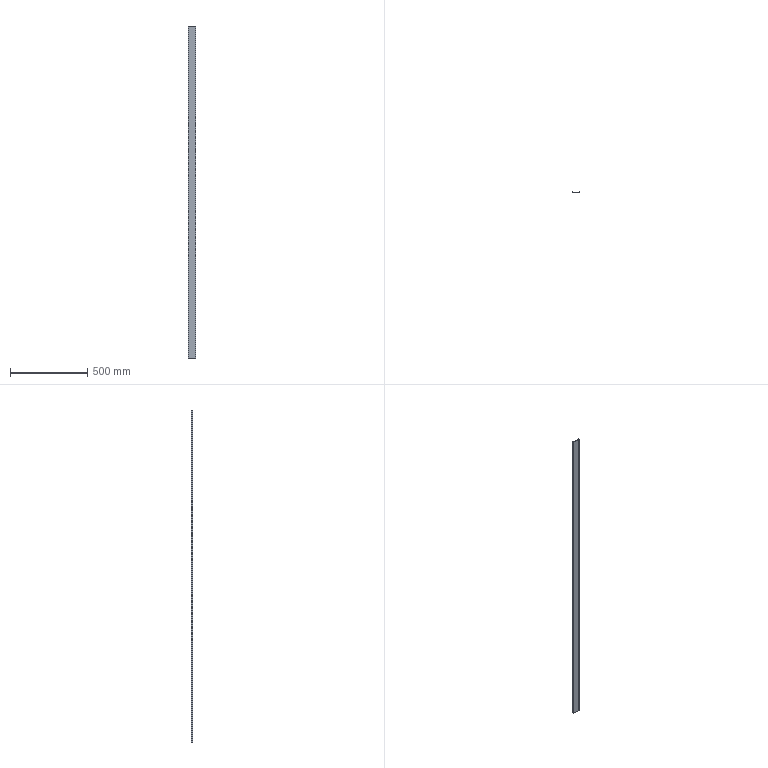Part | STEP file | 31E-01028QY25 | 1 solid | 32 faces | box 50 x 9.195 x 2150 mm | volume 188585 mm3 | cylinder 16 | plane 16 | commonest cylinder face diameters 1 x8 1.2 x6 2 x2
STEP:
#1=CARTESIAN_POINT('',(0.2485,8.595,1075.));
#2=VERTEX_POINT('',#1);
#3=CARTESIAN_POINT('',(0.4243,8.171,1075.));
#4=VERTEX_POINT('',#3);
#5=CARTESIAN_POINT('',(0.8485,8.595,1075.));
#6=DIRECTION('',(0.,0.,-1.));
#7=AXIS2_PLACEMENT_3D('',#5,#6,$);
#8=CIRCLE('',#7,0.6);
#9=EDGE_CURVE('',#2,#4,#8,.F.);
#10=ORIENTED_EDGE('',*,*,#9,.F.);
#11=CARTESIAN_POINT('',(0.2485,8.595,-1075.));
#12=VERTEX_POINT('',#11);
#13=CARTESIAN_POINT('',(0.2485,8.595,1075.));
#14=DIRECTION('',(0.,0.,-1.));
#15=VECTOR('',#14,1.);
#16=LINE('',#13,#15);
#17=EDGE_CURVE('',#2,#12,#16,.T.);
#18=ORIENTED_EDGE('',*,*,#17,.T.);
#19=CARTESIAN_POINT('',(0.4243,8.171,-1075.));
#20=VERTEX_POINT('',#19);
#21=CARTESIAN_POINT('',(0.8485,8.595,-1075.));
#22=DIRECTION('',(0.,0.,-1.));
#23=AXIS2_PLACEMENT_3D('',#21,#22,$);
#24=CIRCLE('',#23,0.6);
#25=EDGE_CURVE('',#20,#12,#24,.T.);
#26=ORIENTED_EDGE('',*,*,#25,.F.);
#27=CARTESIAN_POINT('',(0.4243,8.171,1075.));
#28=DIRECTION('',(0.,0.,-1.));
#29=VECTOR('',#28,1.);
#30=LINE('',#27,#29);
#31=EDGE_CURVE('',#4,#20,#30,.T.);
#32=ORIENTED_EDGE('',*,*,#31,.F.);
#33=EDGE_LOOP('',(#10,#18,#26,#32));
#34=FACE_OUTER_BOUND('',#33,.T.);
#35=CARTESIAN_POINT('',(0.8485,8.595,1075.));
#36=DIRECTION('',(0.,0.,-1.));
#37=DIRECTION('',(1.,0.,0.));
#38=AXIS2_PLACEMENT_3D('',#35,#36,#37);
#39=CYLINDRICAL_SURFACE('',#38,0.6);
#40=ADVANCED_FACE('',(#34),#39,.T.);
#41=CARTESIAN_POINT('',(1.273,9.019,1075.));
#42=VERTEX_POINT('',#41);
#43=CARTESIAN_POINT('',(0.4243,9.019,1075.));
#44=VERTEX_POINT('',#43);
#45=CARTESIAN_POINT('',(1.273,9.019,1075.));
#46=CARTESIAN_POINT('',(1.219,9.073,1075.));
#47=CARTESIAN_POINT('',(1.158,9.118,1075.));
#48=CARTESIAN_POINT('',(1.089,9.152,1075.));
#49=CARTESIAN_POINT('',(0.9442,9.199,1075.));
#50=CARTESIAN_POINT('',(0.7916,9.2,1075.));
#51=CARTESIAN_POINT('',(0.7159,9.188,1075.));
#52=CARTESIAN_POINT('',(0.6071,9.152,1075.));
#53=CARTESIAN_POINT('',(0.5104,9.093,1075.));
#54=CARTESIAN_POINT('',(0.4796,9.07,1075.));
#55=CARTESIAN_POINT('',(0.4509,9.046,1075.));
#56=CARTESIAN_POINT('',(0.4243,9.019,1075.));
#57=B_SPLINE_CURVE_WITH_KNOTS('',5,(#45,#46,#47,#48,#49,#50,#51,#52,#53,#54,#55,#56),.UNSPECIFIED.,.F.,.U.,(6,3,3,6),(0.,0.5331,1.066,1.332),.UNSPECIFIED.);
#58=EDGE_CURVE('',#42,#44,#57,.T.);
#59=ORIENTED_EDGE('',*,*,#58,.T.);
#60=CARTESIAN_POINT('',(0.4243,9.019,1075.));
#61=CARTESIAN_POINT('',(0.3843,8.979,1075.));
#62=CARTESIAN_POINT('',(0.349,8.935,1075.));
#63=CARTESIAN_POINT('',(0.3192,8.886,1075.));
#64=CARTESIAN_POINT('',(0.2795,8.8,1075.));
#65=CARTESIAN_POINT('',(0.2574,8.708,1075.));
#66=CARTESIAN_POINT('',(0.2515,8.67,1075.));
#67=CARTESIAN_POINT('',(0.2485,8.633,1075.));
#68=CARTESIAN_POINT('',(0.2485,8.595,1075.));
#69=B_SPLINE_CURVE_WITH_KNOTS('',5,(#60,#61,#62,#63,#64,#65,#66,#67,#68),.UNSPECIFIED.,.F.,.U.,(6,3,6),(0.,0.3999,0.6659),.UNSPECIFIED.);
#70=EDGE_CURVE('',#44,#2,#69,.T.);
#71=ORIENTED_EDGE('',*,*,#70,.T.);
#72=ORIENTED_EDGE('',*,*,#9,.T.);
#73=CARTESIAN_POINT('',(2.898,5.697,1075.));
#74=VERTEX_POINT('',#73);
#75=CARTESIAN_POINT('',(1.661,6.934,1075.));
#76=DIRECTION('',(0.7071,-0.7071,0.));
#77=VECTOR('',#76,1.);
#78=LINE('',#75,#77);
#79=EDGE_CURVE('',#4,#74,#78,.T.);
#80=ORIENTED_EDGE('',*,*,#79,.T.);
#81=CARTESIAN_POINT('',(0.3706,5.02,1075.));
#82=VERTEX_POINT('',#81);
#83=CARTESIAN_POINT('',(1.634,5.359,1075.));
#84=DIRECTION('',(-0.9659,-0.2588,0.));
#85=VECTOR('',#84,1.);
#86=LINE('',#83,#85);
#87=EDGE_CURVE('',#74,#82,#86,.T.);
#88=ORIENTED_EDGE('',*,*,#87,.T.);
#89=CARTESIAN_POINT('',(0.,4.537,1075.));
#90=VERTEX_POINT('',#89);
#91=CARTESIAN_POINT('',(0.3706,5.02,1075.));
#92=CARTESIAN_POINT('',(0.32,5.007,1075.));
#93=CARTESIAN_POINT('',(0.2712,4.986,1075.));
#94=CARTESIAN_POINT('',(0.2253,4.96,1075.));
#95=CARTESIAN_POINT('',(0.1416,4.896,1075.));
#96=CARTESIAN_POINT('',(0.07725,4.812,1075.));
#97=CARTESIAN_POINT('',(0.05076,4.766,1075.));
#98=CARTESIAN_POINT('',(0.02052,4.693,1075.));
#99=CARTESIAN_POINT('',(0.005155,4.616,1075.));
#100=CARTESIAN_POINT('',(0.001709,4.589,1075.));
#101=CARTESIAN_POINT('',(0.,4.563,1075.));
#102=CARTESIAN_POINT('',(0.,4.537,1075.));
#103=B_SPLINE_CURVE_WITH_KNOTS('',5,(#91,#92,#93,#94,#95,#96,#97,#98,#99,#100,#101,#102),.UNSPECIFIED.,.F.,.U.,(6,3,3,6),(0.,0.3702,0.7405,0.9253),.UNSPECIFIED.);
#104=EDGE_CURVE('',#82,#90,#103,.T.);
#105=ORIENTED_EDGE('',*,*,#104,.T.);
#106=CARTESIAN_POINT('',(0.,1.,1075.));
#107=VERTEX_POINT('',#106);
#108=CARTESIAN_POINT('',(0.,2.769,1075.));
#109=DIRECTION('',(0.,-1.,0.));
#110=VECTOR('',#109,1.);
#111=LINE('',#108,#110);
#112=EDGE_CURVE('',#90,#107,#111,.T.);
#113=ORIENTED_EDGE('',*,*,#112,.T.);
#114=CARTESIAN_POINT('',(1.,0.,1075.));
#115=VERTEX_POINT('',#114);
#116=CARTESIAN_POINT('',(0.,1.,1075.));
#117=CARTESIAN_POINT('',(0.,0.902,1075.));
#118=CARTESIAN_POINT('',(0.012,0.804,1075.));
#119=CARTESIAN_POINT('',(0.036,0.708,1075.));
#120=CARTESIAN_POINT('',(0.107,0.5238,1075.));
#121=CARTESIAN_POINT('',(0.2204,0.3622,1075.));
#122=CARTESIAN_POINT('',(0.2868,0.2888,1075.));
#123=CARTESIAN_POINT('',(0.4361,0.1597,1075.));
#124=CARTESIAN_POINT('',(0.6122,0.0704,1075.));
#125=CARTESIAN_POINT('',(0.7053,0.03682,1075.));
#126=CARTESIAN_POINT('',(0.8215,0.01049,1075.));
#127=CARTESIAN_POINT('',(0.9393,0.001534,1075.));
#128=CARTESIAN_POINT('',(0.9596,0.0005109,1075.));
#129=CARTESIAN_POINT('',(0.9798,0.000000001,1075.));
#130=CARTESIAN_POINT('',(1.,0.000000001,1075.));
#131=B_SPLINE_CURVE_WITH_KNOTS('',5,(#116,#117,#118,#119,#120,#121,#122,#123,#124,#125,#126,#127,#128,#129,#130),.UNSPECIFIED.,.F.,.U.,(6,3,3,3,6),(0.,0.6928,1.386,2.078,2.221),.UNSPECIFIED.);
#132=EDGE_CURVE('',#107,#115,#131,.T.);
#133=ORIENTED_EDGE('',*,*,#132,.T.);
#134=CARTESIAN_POINT('',(49.,0.,1075.));
#135=VERTEX_POINT('',#134);
#136=CARTESIAN_POINT('',(25.,0.000000001,1075.));
#137=DIRECTION('',(1.,0.,0.));
#138=VECTOR('',#137,1.);
#139=LINE('',#136,#138);
#140=EDGE_CURVE('',#115,#135,#139,.T.);
#141=ORIENTED_EDGE('',*,*,#140,.T.);
#142=CARTESIAN_POINT('',(50.,1.,1075.));
#143=VERTEX_POINT('',#142);
#144=CARTESIAN_POINT('',(49.,0.000000001,1075.));
#145=CARTESIAN_POINT('',(49.098,0.000000001,1075.));
#146=CARTESIAN_POINT('',(49.196,0.012,1075.));
#147=CARTESIAN_POINT('',(49.292,0.036,1075.));
#148=CARTESIAN_POINT('',(49.476,0.107,1075.));
#149=CARTESIAN_POINT('',(49.638,0.2204,1075.));
#150=CARTESIAN_POINT('',(49.711,0.2868,1075.));
#151=CARTESIAN_POINT('',(49.84,0.4361,1075.));
#152=CARTESIAN_POINT('',(49.93,0.6122,1075.));
#153=CARTESIAN_POINT('',(49.963,0.7053,1075.));
#154=CARTESIAN_POINT('',(49.99,0.8215,1075.));
#155=CARTESIAN_POINT('',(49.998,0.9393,1075.));
#156=CARTESIAN_POINT('',(49.999,0.9596,1075.));
#157=CARTESIAN_POINT('',(50.,0.9798,1075.));
#158=CARTESIAN_POINT('',(50.,1.,1075.));
#159=B_SPLINE_CURVE_WITH_KNOTS('',5,(#144,#145,#146,#147,#148,#149,#150,#151,#152,#153,#154,#155,#156,#157,#158),.UNSPECIFIED.,.F.,.U.,(6,3,3,3,6),(0.,0.6928,1.386,2.078,2.221),.UNSPECIFIED.);
#160=EDGE_CURVE('',#135,#143,#159,.T.);
#161=ORIENTED_EDGE('',*,*,#160,.T.);
#162=CARTESIAN_POINT('',(50.,4.537,1075.));
#163=VERTEX_POINT('',#162);
#164=CARTESIAN_POINT('',(50.,2.769,1075.));
#165=DIRECTION('',(0.,1.,0.));
#166=VECTOR('',#165,1.);
#167=LINE('',#164,#166);
#168=EDGE_CURVE('',#143,#163,#167,.T.);
#169=ORIENTED_EDGE('',*,*,#168,.T.);
#170=CARTESIAN_POINT('',(49.629,5.02,1075.));
#171=VERTEX_POINT('',#170);
#172=CARTESIAN_POINT('',(50.,4.537,1075.));
#173=CARTESIAN_POINT('',(50.,4.589,1075.));
#174=CARTESIAN_POINT('',(49.993,4.642,1075.));
#175=CARTESIAN_POINT('',(49.979,4.693,1075.));
#176=CARTESIAN_POINT('',(49.939,4.791,1075.));
#177=CARTESIAN_POINT('',(49.875,4.874,1075.));
#178=CARTESIAN_POINT('',(49.837,4.912,1075.));
#179=CARTESIAN_POINT('',(49.774,4.96,1075.));
#180=CARTESIAN_POINT('',(49.704,4.995,1075.));
#181=CARTESIAN_POINT('',(49.679,5.005,1075.));
#182=CARTESIAN_POINT('',(49.655,5.013,1075.));
#183=CARTESIAN_POINT('',(49.629,5.02,1075.));
#184=B_SPLINE_CURVE_WITH_KNOTS('',5,(#172,#173,#174,#175,#176,#177,#178,#179,#180,#181,#182,#183),.UNSPECIFIED.,.F.,.U.,(6,3,3,6),(0.,0.3702,0.7405,0.9253),.UNSPECIFIED.);
#185=EDGE_CURVE('',#163,#171,#184,.T.);
#186=ORIENTED_EDGE('',*,*,#185,.T.);
#187=CARTESIAN_POINT('',(47.102,5.697,1075.));
#188=VERTEX_POINT('',#187);
#189=CARTESIAN_POINT('',(48.366,5.359,1075.));
#190=DIRECTION('',(-0.9659,0.2588,0.));
#191=VECTOR('',#190,1.);
#192=LINE('',#189,#191);
#193=EDGE_CURVE('',#171,#188,#192,.T.);
#194=ORIENTED_EDGE('',*,*,#193,.T.);
#195=CARTESIAN_POINT('',(49.576,8.171,1075.));
#196=VERTEX_POINT('',#195);
#197=CARTESIAN_POINT('',(48.339,6.934,1075.));
#198=DIRECTION('',(0.7071,0.7071,0.));
#199=VECTOR('',#198,1.);
#200=LINE('',#197,#199);
#201=EDGE_CURVE('',#188,#196,#200,.T.);
#202=ORIENTED_EDGE('',*,*,#201,.T.);
#203=CARTESIAN_POINT('',(49.751,8.595,1075.));
#204=VERTEX_POINT('',#203);
#205=CARTESIAN_POINT('',(49.576,8.171,1075.));
#206=CARTESIAN_POINT('',(49.629,8.224,1075.));
#207=CARTESIAN_POINT('',(49.674,8.286,1075.));
#208=CARTESIAN_POINT('',(49.709,8.354,1075.));
#209=CARTESIAN_POINT('',(49.738,8.445,1075.));
#210=CARTESIAN_POINT('',(49.749,8.539,1075.));
#211=CARTESIAN_POINT('',(49.751,8.557,1075.));
#212=CARTESIAN_POINT('',(49.751,8.576,1075.));
#213=CARTESIAN_POINT('',(49.751,8.595,1075.));
#214=B_SPLINE_CURVE_WITH_KNOTS('',5,(#205,#206,#207,#208,#209,#210,#211,#212,#213),.UNSPECIFIED.,.F.,.U.,(6,3,6),(0.,0.5331,0.6664),.UNSPECIFIED.);
#215=EDGE_CURVE('',#196,#204,#214,.T.);
#216=ORIENTED_EDGE('',*,*,#215,.T.);
#217=CARTESIAN_POINT('',(49.576,9.019,1075.));
#218=VERTEX_POINT('',#217);
#219=CARTESIAN_POINT('',(49.751,8.595,1075.));
#220=CARTESIAN_POINT('',(49.751,8.652,1075.));
#221=CARTESIAN_POINT('',(49.745,8.708,1075.));
#222=CARTESIAN_POINT('',(49.731,8.764,1075.));
#223=CARTESIAN_POINT('',(49.699,8.853,1075.));
#224=CARTESIAN_POINT('',(49.649,8.933,1075.));
#225=CARTESIAN_POINT('',(49.627,8.964,1075.));
#226=CARTESIAN_POINT('',(49.602,8.993,1075.));
#227=CARTESIAN_POINT('',(49.576,9.019,1075.));
#228=B_SPLINE_CURVE_WITH_KNOTS('',5,(#219,#220,#221,#222,#223,#224,#225,#226,#227),.UNSPECIFIED.,.F.,.U.,(6,3,6),(0.6664,1.066,1.332),.UNSPECIFIED.);
#229=EDGE_CURVE('',#204,#218,#228,.T.);
#230=ORIENTED_EDGE('',*,*,#229,.T.);
#231=CARTESIAN_POINT('',(48.727,9.019,1075.));
#232=VERTEX_POINT('',#231);
#233=CARTESIAN_POINT('',(49.576,9.019,1075.));
#234=CARTESIAN_POINT('',(49.522,9.073,1075.));
#235=CARTESIAN_POINT('',(49.461,9.118,1075.));
#236=CARTESIAN_POINT('',(49.392,9.152,1075.));
#237=CARTESIAN_POINT('',(49.247,9.199,1075.));
#238=CARTESIAN_POINT('',(49.095,9.2,1075.));
#239=CARTESIAN_POINT('',(49.019,9.188,1075.));
#240=CARTESIAN_POINT('',(48.91,9.152,1075.));
#241=CARTESIAN_POINT('',(48.813,9.093,1075.));
#242=CARTESIAN_POINT('',(48.782,9.07,1075.));
#243=CARTESIAN_POINT('',(48.754,9.046,1075.));
#244=CARTESIAN_POINT('',(48.727,9.019,1075.));
#245=B_SPLINE_CURVE_WITH_KNOTS('',5,(#233,#234,#235,#236,#237,#238,#239,#240,#241,#242,#243,#244),.UNSPECIFIED.,.F.,.U.,(6,3,3,6),(0.,0.5331,1.066,1.332),.UNSPECIFIED.);
#246=EDGE_CURVE('',#218,#232,#245,.T.);
#247=ORIENTED_EDGE('',*,*,#246,.T.);
#248=CARTESIAN_POINT('',(45.396,5.688,1075.));
#249=VERTEX_POINT('',#248);
#250=CARTESIAN_POINT('',(47.062,7.354,1075.));
#251=DIRECTION('',(-0.7071,-0.7071,0.));
#252=VECTOR('',#251,1.);
#253=LINE('',#250,#252);
#254=EDGE_CURVE('',#232,#249,#253,.T.);
#255=ORIENTED_EDGE('',*,*,#254,.T.);
#256=CARTESIAN_POINT('',(45.25,5.335,1075.));
#257=VERTEX_POINT('',#256);
#258=CARTESIAN_POINT('',(45.396,5.688,1075.));
#259=CARTESIAN_POINT('',(45.363,5.655,1075.));
#260=CARTESIAN_POINT('',(45.334,5.618,1075.));
#261=CARTESIAN_POINT('',(45.309,5.577,1075.));
#262=CARTESIAN_POINT('',(45.276,5.506,1075.));
#263=CARTESIAN_POINT('',(45.257,5.429,1075.));
#264=CARTESIAN_POINT('',(45.252,5.398,1075.));
#265=CARTESIAN_POINT('',(45.25,5.366,1075.));
#266=CARTESIAN_POINT('',(45.25,5.335,1075.));
#267=B_SPLINE_CURVE_WITH_KNOTS('',5,(#258,#259,#260,#261,#262,#263,#264,#265,#266),.UNSPECIFIED.,.F.,.U.,(6,3,6),(0.,0.3332,0.5549),.UNSPECIFIED.);
#268=EDGE_CURVE('',#249,#257,#267,.T.);
#269=ORIENTED_EDGE('',*,*,#268,.T.);
#270=CARTESIAN_POINT('',(45.621,4.852,1075.));
#271=VERTEX_POINT('',#270);
#272=CARTESIAN_POINT('',(45.25,5.335,1075.));
#273=CARTESIAN_POINT('',(45.25,5.283,1075.));
#274=CARTESIAN_POINT('',(45.257,5.23,1075.));
#275=CARTESIAN_POINT('',(45.27,5.179,1075.));
#276=CARTESIAN_POINT('',(45.311,5.081,1075.));
#277=CARTESIAN_POINT('',(45.375,4.998,1075.));
#278=CARTESIAN_POINT('',(45.413,4.96,1075.));
#279=CARTESIAN_POINT('',(45.476,4.912,1075.));
#280=CARTESIAN_POINT('',(45.546,4.877,1075.));
#281=CARTESIAN_POINT('',(45.57,4.867,1075.));
#282=CARTESIAN_POINT('',(45.595,4.859,1075.));
#283=CARTESIAN_POINT('',(45.621,4.852,1075.));
#284=B_SPLINE_CURVE_WITH_KNOTS('',5,(#272,#273,#274,#275,#276,#277,#278,#279,#280,#281,#282,#283),.UNSPECIFIED.,.F.,.U.,(6,3,3,6),(0.,0.3702,0.7405,0.9253),.UNSPECIFIED.);
#285=EDGE_CURVE('',#257,#271,#284,.T.);
#286=ORIENTED_EDGE('',*,*,#285,.T.);
#287=CARTESIAN_POINT('',(48.8,4.,1075.));
#288=VERTEX_POINT('',#287);
#289=CARTESIAN_POINT('',(47.21,4.426,1075.));
#290=DIRECTION('',(0.9659,-0.2588,0.));
#291=VECTOR('',#290,1.);
#292=LINE('',#289,#291);
#293=EDGE_CURVE('',#271,#288,#292,.T.);
#294=ORIENTED_EDGE('',*,*,#293,.T.);
#295=CARTESIAN_POINT('',(48.8,1.7,1075.));
#296=VERTEX_POINT('',#295);
#297=CARTESIAN_POINT('',(48.8,2.85,1075.));
#298=DIRECTION('',(0.,-1.,0.));
#299=VECTOR('',#298,1.);
#300=LINE('',#297,#299);
#301=EDGE_CURVE('',#288,#296,#300,.T.);
#302=ORIENTED_EDGE('',*,*,#301,.T.);
#303=CARTESIAN_POINT('',(48.3,1.2,1075.));
#304=VERTEX_POINT('',#303);
#305=CARTESIAN_POINT('',(48.3,1.7,1075.));
#306=DIRECTION('',(0.,0.,-1.));
#307=AXIS2_PLACEMENT_3D('',#305,#306,$);
#308=CIRCLE('',#307,0.5);
#309=EDGE_CURVE('',#296,#304,#308,.T.);
#310=ORIENTED_EDGE('',*,*,#309,.T.);
#311=CARTESIAN_POINT('',(1.7,1.2,1075.));
#312=VERTEX_POINT('',#311);
#313=CARTESIAN_POINT('',(25.,1.2,1075.));
#314=DIRECTION('',(-1.,0.,0.));
#315=VECTOR('',#314,1.);
#316=LINE('',#313,#315);
#317=EDGE_CURVE('',#304,#312,#316,.T.);
#318=ORIENTED_EDGE('',*,*,#317,.T.);
#319=CARTESIAN_POINT('',(1.2,1.7,1075.));
#320=VERTEX_POINT('',#319);
#321=CARTESIAN_POINT('',(1.7,1.7,1075.));
#322=DIRECTION('',(0.,0.,-1.));
#323=AXIS2_PLACEMENT_3D('',#321,#322,$);
#324=CIRCLE('',#323,0.5);
#325=EDGE_CURVE('',#312,#320,#324,.T.);
#326=ORIENTED_EDGE('',*,*,#325,.T.);
#327=CARTESIAN_POINT('',(1.2,4.,1075.));
#328=VERTEX_POINT('',#327);
#329=CARTESIAN_POINT('',(1.2,2.85,1075.));
#330=DIRECTION('',(0.,1.,0.));
#331=VECTOR('',#330,1.);
#332=LINE('',#329,#331);
#333=EDGE_CURVE('',#320,#328,#332,.T.);
#334=ORIENTED_EDGE('',*,*,#333,.T.);
#335=CARTESIAN_POINT('',(4.379,4.852,1075.));
#336=VERTEX_POINT('',#335);
#337=CARTESIAN_POINT('',(2.79,4.426,1075.));
#338=DIRECTION('',(0.9659,0.2588,0.));
#339=VECTOR('',#338,1.);
#340=LINE('',#337,#339);
#341=EDGE_CURVE('',#328,#336,#340,.T.);
#342=ORIENTED_EDGE('',*,*,#341,.T.);
#343=CARTESIAN_POINT('',(4.75,5.335,1075.));
#344=VERTEX_POINT('',#343);
#345=CARTESIAN_POINT('',(4.379,4.852,1075.));
#346=CARTESIAN_POINT('',(4.446,4.87,1075.));
#347=CARTESIAN_POINT('',(4.51,4.899,1075.));
#348=CARTESIAN_POINT('',(4.568,4.94,1075.));
#349=CARTESIAN_POINT('',(4.662,5.034,1075.));
#350=CARTESIAN_POINT('',(4.722,5.152,1075.));
#351=CARTESIAN_POINT('',(4.741,5.212,1075.));
#352=CARTESIAN_POINT('',(4.75,5.273,1075.));
#353=CARTESIAN_POINT('',(4.75,5.335,1075.));
#354=B_SPLINE_CURVE_WITH_KNOTS('',5,(#345,#346,#347,#348,#349,#350,#351,#352,#353),.UNSPECIFIED.,.F.,.U.,(6,3,6),(0.,0.4899,0.9256),.UNSPECIFIED.);
#355=EDGE_CURVE('',#336,#344,#354,.T.);
#356=ORIENTED_EDGE('',*,*,#355,.T.);
#357=CARTESIAN_POINT('',(4.604,5.688,1075.));
#358=VERTEX_POINT('',#357);
#359=CARTESIAN_POINT('',(4.75,5.335,1075.));
#360=CARTESIAN_POINT('',(4.75,5.343,1075.));
#361=CARTESIAN_POINT('',(4.75,5.35,1075.));
#362=CARTESIAN_POINT('',(4.75,5.358,1075.));
#363=CARTESIAN_POINT('',(4.745,5.435,1075.));
#364=CARTESIAN_POINT('',(4.726,5.51,1075.));
#365=CARTESIAN_POINT('',(4.697,5.575,1075.));
#366=CARTESIAN_POINT('',(4.657,5.634,1075.));
#367=CARTESIAN_POINT('',(4.607,5.685,1075.));
#368=CARTESIAN_POINT('',(4.606,5.686,1075.));
#369=CARTESIAN_POINT('',(4.605,5.687,1075.));
#370=CARTESIAN_POINT('',(4.604,5.688,1075.));
#371=B_SPLINE_CURVE_WITH_KNOTS('',5,(#359,#360,#361,#362,#363,#364,#365,#366,#367,#368,#369,#370),.UNSPECIFIED.,.F.,.U.,(6,3,3,6),(0.9256,0.9798,1.47,1.481),.UNSPECIFIED.);
#372=EDGE_CURVE('',#344,#358,#371,.T.);
#373=ORIENTED_EDGE('',*,*,#372,.T.);
#374=CARTESIAN_POINT('',(2.938,7.354,1075.));
#375=DIRECTION('',(-0.7071,0.7071,0.));
#376=VECTOR('',#375,1.);
#377=LINE('',#374,#376);
#378=EDGE_CURVE('',#358,#42,#377,.T.);
#379=ORIENTED_EDGE('',*,*,#378,.T.);
#380=EDGE_LOOP('',(#59,#71,#72,#80,#88,#105,#113,#133,#141,#161,#169,#186,#194,#202,#216,#230,#247,#255,#269,#286,#294,#302,#310,#318,#326,#334,#342,#356,#373,#379));
#381=FACE_OUTER_BOUND('',#380,.T.);
#382=CARTESIAN_POINT('',(0.,1.2,1075.));
#383=DIRECTION('',(0.,0.,-1.));
#384=DIRECTION('',(-1.,0.,0.));
#385=AXIS2_PLACEMENT_3D('',#382,#383,#384);
#386=PLANE('',#385);
#387=ADVANCED_FACE('',(#381),#386,.F.);
#388=ORIENTED_EDGE('',*,*,#17,.F.);
#389=ORIENTED_EDGE('',*,*,#70,.F.);
#390=CARTESIAN_POINT('',(0.4243,9.019,-1075.));
#391=VERTEX_POINT('',#390);
#392=CARTESIAN_POINT('',(0.4243,9.019,1075.));
#393=DIRECTION('',(0.,0.,-1.));
#394=VECTOR('',#393,1.);
#395=LINE('',#392,#394);
#396=EDGE_CURVE('',#44,#391,#395,.T.);
#397=ORIENTED_EDGE('',*,*,#396,.T.);
#398=CARTESIAN_POINT('',(0.8485,8.595,-1075.));
#399=DIRECTION('',(0.,0.,-1.));
#400=AXIS2_PLACEMENT_3D('',#398,#399,$);
#401=CIRCLE('',#400,0.6);
#402=EDGE_CURVE('',#12,#391,#401,.T.);
#403=ORIENTED_EDGE('',*,*,#402,.F.);
#404=EDGE_LOOP('',(#388,#389,#397,#403));
#405=FACE_OUTER_BOUND('',#404,.T.);
#406=CARTESIAN_POINT('',(0.8485,8.595,1075.));
#407=DIRECTION('',(0.,0.,-1.));
#408=DIRECTION('',(-1.,0.,0.));
#409=AXIS2_PLACEMENT_3D('',#406,#407,#408);
#410=CYLINDRICAL_SURFACE('',#409,0.6);
#411=ADVANCED_FACE('',(#405),#410,.T.);
#412=CARTESIAN_POINT('',(2.898,5.697,-1075.));
#413=VERTEX_POINT('',#412);
#414=CARTESIAN_POINT('',(1.661,6.934,-1075.));
#415=DIRECTION('',(0.7071,-0.7071,0.));
#416=VECTOR('',#415,1.);
#417=LINE('',#414,#416);
#418=EDGE_CURVE('',#20,#413,#417,.T.);
#419=ORIENTED_EDGE('',*,*,#418,.F.);
#420=ORIENTED_EDGE('',*,*,#25,.T.);
#421=ORIENTED_EDGE('',*,*,#402,.T.);
#422=CARTESIAN_POINT('',(1.273,9.019,-1075.));
#423=VERTEX_POINT('',#422);
#424=CARTESIAN_POINT('',(0.8485,8.595,-1075.));
#425=DIRECTION('',(0.,0.,-1.));
#426=AXIS2_PLACEMENT_3D('',#424,#425,$);
#427=CIRCLE('',#426,0.6);
#428=EDGE_CURVE('',#391,#423,#427,.T.);
#429=ORIENTED_EDGE('',*,*,#428,.T.);
#430=CARTESIAN_POINT('',(4.604,5.688,-1075.));
#431=VERTEX_POINT('',#430);
#432=CARTESIAN_POINT('',(2.938,7.354,-1075.));
#433=DIRECTION('',(-0.7071,0.7071,0.));
#434=VECTOR('',#433,1.);
#435=LINE('',#432,#434);
#436=EDGE_CURVE('',#431,#423,#435,.T.);
#437=ORIENTED_EDGE('',*,*,#436,.F.);
#438=CARTESIAN_POINT('',(4.75,5.335,-1075.));
#439=VERTEX_POINT('',#438);
#440=CARTESIAN_POINT('',(4.25,5.335,-1075.));
#441=DIRECTION('',(0.,0.,-1.));
#442=AXIS2_PLACEMENT_3D('',#440,#441,$);
#443=CIRCLE('',#442,0.5);
#444=EDGE_CURVE('',#431,#439,#443,.T.);
#445=ORIENTED_EDGE('',*,*,#444,.T.);
#446=CARTESIAN_POINT('',(4.379,4.852,-1075.));
#447=VERTEX_POINT('',#446);
#448=CARTESIAN_POINT('',(4.25,5.335,-1075.));
#449=DIRECTION('',(0.,0.,-1.));
#450=AXIS2_PLACEMENT_3D('',#448,#449,$);
#451=CIRCLE('',#450,0.5);
#452=EDGE_CURVE('',#439,#447,#451,.T.);
#453=ORIENTED_EDGE('',*,*,#452,.T.);
#454=CARTESIAN_POINT('',(1.2,4.,-1075.));
#455=VERTEX_POINT('',#454);
#456=CARTESIAN_POINT('',(2.79,4.426,-1075.));
#457=DIRECTION('',(0.9659,0.2588,0.));
#458=VECTOR('',#457,1.);
#459=LINE('',#456,#458);
#460=EDGE_CURVE('',#455,#447,#459,.T.);
#461=ORIENTED_EDGE('',*,*,#460,.F.);
#462=CARTESIAN_POINT('',(1.2,1.7,-1075.));
#463=VERTEX_POINT('',#462);
#464=CARTESIAN_POINT('',(1.2,2.85,-1075.));
#465=DIRECTION('',(0.,1.,0.));
#466=VECTOR('',#465,1.);
#467=LINE('',#464,#466);
#468=EDGE_CURVE('',#463,#455,#467,.T.);
#469=ORIENTED_EDGE('',*,*,#468,.F.);
#470=CARTESIAN_POINT('',(1.7,1.2,-1075.));
#471=VERTEX_POINT('',#470);
#472=CARTESIAN_POINT('',(1.2,1.7,-1075.));
#473=CARTESIAN_POINT('',(1.2,1.637,-1075.));
#474=CARTESIAN_POINT('',(1.21,1.574,-1075.));
#475=CARTESIAN_POINT('',(1.23,1.514,-1075.));
#476=CARTESIAN_POINT('',(1.288,1.4,-1075.));
#477=CARTESIAN_POINT('',(1.377,1.31,-1075.));
#478=CARTESIAN_POINT('',(1.429,1.273,-1075.));
#479=CARTESIAN_POINT('',(1.514,1.23,-1075.));
#480=CARTESIAN_POINT('',(1.606,1.207,-1075.));
#481=CARTESIAN_POINT('',(1.637,1.202,-1075.));
#482=CARTESIAN_POINT('',(1.669,1.2,-1075.));
#483=CARTESIAN_POINT('',(1.7,1.2,-1075.));
#484=B_SPLINE_CURVE_WITH_KNOTS('',5,(#472,#473,#474,#475,#476,#477,#478,#479,#480,#481,#482,#483),.UNSPECIFIED.,.F.,.U.,(6,3,3,6),(0.,0.4443,0.8886,1.11),.UNSPECIFIED.);
#485=EDGE_CURVE('',#463,#471,#484,.T.);
#486=ORIENTED_EDGE('',*,*,#485,.T.);
#487=CARTESIAN_POINT('',(48.3,1.2,-1075.));
#488=VERTEX_POINT('',#487);
#489=CARTESIAN_POINT('',(25.,1.2,-1075.));
#490=DIRECTION('',(-1.,0.,0.));
#491=VECTOR('',#490,1.);
#492=LINE('',#489,#491);
#493=EDGE_CURVE('',#488,#471,#492,.T.);
#494=ORIENTED_EDGE('',*,*,#493,.F.);
#495=CARTESIAN_POINT('',(48.8,1.7,-1075.));
#496=VERTEX_POINT('',#495);
#497=CARTESIAN_POINT('',(48.3,1.2,-1075.));
#498=CARTESIAN_POINT('',(48.363,1.2,-1075.));
#499=CARTESIAN_POINT('',(48.426,1.21,-1075.));
#500=CARTESIAN_POINT('',(48.486,1.23,-1075.));
#501=CARTESIAN_POINT('',(48.6,1.288,-1075.));
#502=CARTESIAN_POINT('',(48.69,1.377,-1075.));
#503=CARTESIAN_POINT('',(48.727,1.429,-1075.));
#504=CARTESIAN_POINT('',(48.77,1.514,-1075.));
#505=CARTESIAN_POINT('',(48.793,1.606,-1075.));
#506=CARTESIAN_POINT('',(48.798,1.637,-1075.));
#507=CARTESIAN_POINT('',(48.8,1.669,-1075.));
#508=CARTESIAN_POINT('',(48.8,1.7,-1075.));
#509=B_SPLINE_CURVE_WITH_KNOTS('',5,(#497,#498,#499,#500,#501,#502,#503,#504,#505,#506,#507,#508),.UNSPECIFIED.,.F.,.U.,(6,3,3,6),(0.,0.4443,0.8886,1.11),.UNSPECIFIED.);
#510=EDGE_CURVE('',#488,#496,#509,.T.);
#511=ORIENTED_EDGE('',*,*,#510,.T.);
#512=CARTESIAN_POINT('',(48.8,4.,-1075.));
#513=VERTEX_POINT('',#512);
#514=CARTESIAN_POINT('',(48.8,2.85,-1075.));
#515=DIRECTION('',(0.,-1.,0.));
#516=VECTOR('',#515,1.);
#517=LINE('',#514,#516);
#518=EDGE_CURVE('',#513,#496,#517,.T.);
#519=ORIENTED_EDGE('',*,*,#518,.F.);
#520=CARTESIAN_POINT('',(45.621,4.852,-1075.));
#521=VERTEX_POINT('',#520);
#522=CARTESIAN_POINT('',(47.21,4.426,-1075.));
#523=DIRECTION('',(0.9659,-0.2588,0.));
#524=VECTOR('',#523,1.);
#525=LINE('',#522,#524);
#526=EDGE_CURVE('',#521,#513,#525,.T.);
#527=ORIENTED_EDGE('',*,*,#526,.F.);
#528=CARTESIAN_POINT('',(45.25,5.335,-1075.));
#529=VERTEX_POINT('',#528);
#530=CARTESIAN_POINT('',(45.75,5.335,-1075.));
#531=DIRECTION('',(0.,0.,-1.));
#532=AXIS2_PLACEMENT_3D('',#530,#531,$);
#533=CIRCLE('',#532,0.5);
#534=EDGE_CURVE('',#521,#529,#533,.T.);
#535=ORIENTED_EDGE('',*,*,#534,.T.);
#536=CARTESIAN_POINT('',(45.396,5.688,-1075.));
#537=VERTEX_POINT('',#536);
#538=CARTESIAN_POINT('',(45.75,5.335,-1075.));
#539=DIRECTION('',(0.,0.,-1.));
#540=AXIS2_PLACEMENT_3D('',#538,#539,$);
#541=CIRCLE('',#540,0.5);
#542=EDGE_CURVE('',#529,#537,#541,.T.);
#543=ORIENTED_EDGE('',*,*,#542,.T.);
#544=CARTESIAN_POINT('',(48.727,9.019,-1075.));
#545=VERTEX_POINT('',#544);
#546=CARTESIAN_POINT('',(47.062,7.354,-1075.));
#547=DIRECTION('',(-0.7071,-0.7071,0.));
#548=VECTOR('',#547,1.);
#549=LINE('',#546,#548);
#550=EDGE_CURVE('',#545,#537,#549,.T.);
#551=ORIENTED_EDGE('',*,*,#550,.F.);
#552=CARTESIAN_POINT('',(49.576,9.019,-1075.));
#553=VERTEX_POINT('',#552);
#554=CARTESIAN_POINT('',(49.151,8.595,-1075.));
#555=DIRECTION('',(0.,0.,-1.));
#556=AXIS2_PLACEMENT_3D('',#554,#555,$);
#557=CIRCLE('',#556,0.6);
#558=EDGE_CURVE('',#545,#553,#557,.T.);
#559=ORIENTED_EDGE('',*,*,#558,.T.);
#560=CARTESIAN_POINT('',(49.751,8.595,-1075.));
#561=VERTEX_POINT('',#560);
#562=CARTESIAN_POINT('',(49.151,8.595,-1075.));
#563=DIRECTION('',(0.,0.,-1.));
#564=AXIS2_PLACEMENT_3D('',#562,#563,$);
#565=CIRCLE('',#564,0.6);
#566=EDGE_CURVE('',#553,#561,#565,.T.);
#567=ORIENTED_EDGE('',*,*,#566,.T.);
#568=CARTESIAN_POINT('',(49.576,8.171,-1075.));
#569=VERTEX_POINT('',#568);
#570=CARTESIAN_POINT('',(49.151,8.595,-1075.));
#571=DIRECTION('',(0.,0.,-1.));
#572=AXIS2_PLACEMENT_3D('',#570,#571,$);
#573=CIRCLE('',#572,0.6);
#574=EDGE_CURVE('',#561,#569,#573,.T.);
#575=ORIENTED_EDGE('',*,*,#574,.T.);
#576=CARTESIAN_POINT('',(47.102,5.697,-1075.));
#577=VERTEX_POINT('',#576);
#578=CARTESIAN_POINT('',(48.339,6.934,-1075.));
#579=DIRECTION('',(0.7071,0.7071,0.));
#580=VECTOR('',#579,1.);
#581=LINE('',#578,#580);
#582=EDGE_CURVE('',#577,#569,#581,.T.);
#583=ORIENTED_EDGE('',*,*,#582,.F.);
#584=CARTESIAN_POINT('',(49.629,5.02,-1075.));
#585=VERTEX_POINT('',#584);
#586=CARTESIAN_POINT('',(48.366,5.359,-1075.));
#587=DIRECTION('',(-0.9659,0.2588,0.));
#588=VECTOR('',#587,1.);
#589=LINE('',#586,#588);
#590=EDGE_CURVE('',#585,#577,#589,.T.);
#591=ORIENTED_EDGE('',*,*,#590,.F.);
#592=CARTESIAN_POINT('',(50.,4.537,-1075.));
#593=VERTEX_POINT('',#592);
#594=CARTESIAN_POINT('',(49.5,4.537,-1075.));
#595=DIRECTION('',(0.,0.,-1.));
#596=AXIS2_PLACEMENT_3D('',#594,#595,$);
#597=CIRCLE('',#596,0.5);
#598=EDGE_CURVE('',#585,#593,#597,.T.);
#599=ORIENTED_EDGE('',*,*,#598,.T.);
#600=CARTESIAN_POINT('',(50.,1.,-1075.));
#601=VERTEX_POINT('',#600);
#602=CARTESIAN_POINT('',(50.,2.769,-1075.));
#603=DIRECTION('',(0.,1.,0.));
#604=VECTOR('',#603,1.);
#605=LINE('',#602,#604);
#606=EDGE_CURVE('',#601,#593,#605,.T.);
#607=ORIENTED_EDGE('',*,*,#606,.F.);
#608=CARTESIAN_POINT('',(49.,0.,-1075.));
#609=VERTEX_POINT('',#608);
#610=CARTESIAN_POINT('',(49.,1.,-1075.));
#611=DIRECTION('',(0.,0.,-1.));
#612=AXIS2_PLACEMENT_3D('',#610,#611,$);
#613=CIRCLE('',#612,1.);
#614=EDGE_CURVE('',#601,#609,#613,.T.);
#615=ORIENTED_EDGE('',*,*,#614,.T.);
#616=CARTESIAN_POINT('',(1.,0.,-1075.));
#617=VERTEX_POINT('',#616);
#618=CARTESIAN_POINT('',(25.,0.000000001,-1075.));
#619=DIRECTION('',(1.,0.,0.));
#620=VECTOR('',#619,1.);
#621=LINE('',#618,#620);
#622=EDGE_CURVE('',#617,#609,#621,.T.);
#623=ORIENTED_EDGE('',*,*,#622,.F.);
#624=CARTESIAN_POINT('',(0.,1.,-1075.));
#625=VERTEX_POINT('',#624);
#626=CARTESIAN_POINT('',(1.,1.,-1075.));
#627=DIRECTION('',(0.,0.,-1.));
#628=AXIS2_PLACEMENT_3D('',#626,#627,$);
#629=CIRCLE('',#628,1.);
#630=EDGE_CURVE('',#617,#625,#629,.T.);
#631=ORIENTED_EDGE('',*,*,#630,.T.);
#632=CARTESIAN_POINT('',(0.,4.537,-1075.));
#633=VERTEX_POINT('',#632);
#634=CARTESIAN_POINT('',(0.,2.769,-1075.));
#635=DIRECTION('',(0.,-1.,0.));
#636=VECTOR('',#635,1.);
#637=LINE('',#634,#636);
#638=EDGE_CURVE('',#633,#625,#637,.T.);
#639=ORIENTED_EDGE('',*,*,#638,.F.);
#640=CARTESIAN_POINT('',(0.3706,5.02,-1075.));
#641=VERTEX_POINT('',#640);
#642=CARTESIAN_POINT('',(0.5,4.537,-1075.));
#643=DIRECTION('',(0.,0.,-1.));
#644=AXIS2_PLACEMENT_3D('',#642,#643,$);
#645=CIRCLE('',#644,0.5);
#646=EDGE_CURVE('',#633,#641,#645,.T.);
#647=ORIENTED_EDGE('',*,*,#646,.T.);
#648=CARTESIAN_POINT('',(1.634,5.359,-1075.));
#649=DIRECTION('',(-0.9659,-0.2588,0.));
#650=VECTOR('',#649,1.);
#651=LINE('',#648,#650);
#652=EDGE_CURVE('',#413,#641,#651,.T.);
#653=ORIENTED_EDGE('',*,*,#652,.F.);
#654=EDGE_LOOP('',(#419,#420,#421,#429,#437,#445,#453,#461,#469,#486,#494,#511,#519,#527,#535,#543,#551,#559,#567,#575,#583,#591,#599,#607,#615,#623,#631,#639,#647,#653));
#655=FACE_OUTER_BOUND('',#654,.T.);
#656=CARTESIAN_POINT('',(0.,1.2,-1075.));
#657=DIRECTION('',(0.,0.,-1.));
#658=DIRECTION('',(-1.,0.,0.));
#659=AXIS2_PLACEMENT_3D('',#656,#657,#658);
#660=PLANE('',#659);
#661=ADVANCED_FACE('',(#655),#660,.T.);
#662=ORIENTED_EDGE('',*,*,#79,.F.);
#663=ORIENTED_EDGE('',*,*,#31,.T.);
#664=ORIENTED_EDGE('',*,*,#418,.T.);
#665=CARTESIAN_POINT('',(2.898,5.697,0.));
#666=DIRECTION('',(0.,0.,-1.));
#667=VECTOR('',#666,1.);
#668=LINE('',#665,#667);
#669=EDGE_CURVE('',#74,#413,#668,.T.);
#670=ORIENTED_EDGE('',*,*,#669,.F.);
#671=EDGE_LOOP('',(#662,#663,#664,#670));
#672=FACE_OUTER_BOUND('',#671,.T.);
#673=CARTESIAN_POINT('',(2.898,5.697,1075.));
#674=DIRECTION('',(0.7071,0.7071,0.));
#675=DIRECTION('',(-0.7071,0.7071,0.));
#676=AXIS2_PLACEMENT_3D('',#673,#674,#675);
#677=PLANE('',#676);
#678=ADVANCED_FACE('',(#672),#677,.F.);
#679=ORIENTED_EDGE('',*,*,#396,.F.);
#680=ORIENTED_EDGE('',*,*,#58,.F.);
#681=CARTESIAN_POINT('',(1.273,9.019,1075.));
#682=DIRECTION('',(0.,0.,-1.));
#683=VECTOR('',#682,1.);
#684=LINE('',#681,#683);
#685=EDGE_CURVE('',#423,#42,#684,.F.);
#686=ORIENTED_EDGE('',*,*,#685,.F.);
#687=ORIENTED_EDGE('',*,*,#428,.F.);
#688=EDGE_LOOP('',(#679,#680,#686,#687));
#689=FACE_OUTER_BOUND('',#688,.T.);
#690=CARTESIAN_POINT('',(0.8485,8.595,1075.));
#691=DIRECTION('',(0.,0.,-1.));
#692=DIRECTION('',(-1.,0.,0.));
#693=AXIS2_PLACEMENT_3D('',#690,#691,#692);
#694=CYLINDRICAL_SURFACE('',#693,0.6);
#695=ADVANCED_FACE('',(#689),#694,.T.);
#696=ORIENTED_EDGE('',*,*,#652,.T.);
#697=CARTESIAN_POINT('',(0.3706,5.02,0.));
#698=DIRECTION('',(0.,0.,1.));
#699=VECTOR('',#698,1.);
#700=LINE('',#697,#699);
#701=EDGE_CURVE('',#641,#82,#700,.T.);
#702=ORIENTED_EDGE('',*,*,#701,.T.);
#703=ORIENTED_EDGE('',*,*,#87,.F.);
#704=ORIENTED_EDGE('',*,*,#669,.T.);
#705=EDGE_LOOP('',(#696,#702,#703,#704));
#706=FACE_OUTER_BOUND('',#705,.T.);
#707=CARTESIAN_POINT('',(0.,4.921,1075.));
#708=DIRECTION('',(0.2588,-0.9659,0.));
#709=DIRECTION('',(0.9659,0.2588,0.));
#710=AXIS2_PLACEMENT_3D('',#707,#708,#709);
#711=PLANE('',#710);
#712=ADVANCED_FACE('',(#706),#711,.F.);
#713=ORIENTED_EDGE('',*,*,#104,.F.);
#714=ORIENTED_EDGE('',*,*,#701,.F.);
#715=ORIENTED_EDGE('',*,*,#646,.F.);
#716=CARTESIAN_POINT('',(0.,4.537,1075.));
#717=DIRECTION('',(0.,0.,-1.));
#718=VECTOR('',#717,1.);
#719=LINE('',#716,#718);
#720=EDGE_CURVE('',#90,#633,#719,.T.);
#721=ORIENTED_EDGE('',*,*,#720,.F.);
#722=EDGE_LOOP('',(#713,#714,#715,#721));
#723=FACE_OUTER_BOUND('',#722,.T.);
#724=CARTESIAN_POINT('',(0.5,4.537,1075.));
#725=DIRECTION('',(0.,0.,-1.));
#726=DIRECTION('',(-1.,0.,0.));
#727=AXIS2_PLACEMENT_3D('',#724,#725,#726);
#728=CYLINDRICAL_SURFACE('',#727,0.5);
#729=ADVANCED_FACE('',(#723),#728,.T.);
#730=ORIENTED_EDGE('',*,*,#112,.F.);
#731=ORIENTED_EDGE('',*,*,#720,.T.);
#732=ORIENTED_EDGE('',*,*,#638,.T.);
#733=CARTESIAN_POINT('',(0.,1.,0.));
#734=DIRECTION('',(0.,0.,1.));
#735=VECTOR('',#734,1.);
#736=LINE('',#733,#735);
#737=EDGE_CURVE('',#625,#107,#736,.T.);
#738=ORIENTED_EDGE('',*,*,#737,.T.);
#739=EDGE_LOOP('',(#730,#731,#732,#738));
#740=FACE_OUTER_BOUND('',#739,.T.);
#741=CARTESIAN_POINT('',(0.,0.,1075.));
#742=DIRECTION('',(1.,0.,0.));
#743=DIRECTION('',(0.,1.,0.));
#744=AXIS2_PLACEMENT_3D('',#741,#742,#743);
#745=PLANE('',#744);
#746=ADVANCED_FACE('',(#740),#745,.F.);
#747=ORIENTED_EDGE('',*,*,#132,.F.);
#748=ORIENTED_EDGE('',*,*,#737,.F.);
#749=ORIENTED_EDGE('',*,*,#630,.F.);
#750=CARTESIAN_POINT('',(1.,0.,1075.));
#751=DIRECTION('',(0.,0.,-1.));
#752=VECTOR('',#751,1.);
#753=LINE('',#750,#752);
#754=EDGE_CURVE('',#115,#617,#753,.T.);
#755=ORIENTED_EDGE('',*,*,#754,.F.);
#756=EDGE_LOOP('',(#747,#748,#749,#755));
#757=FACE_OUTER_BOUND('',#756,.T.);
#758=CARTESIAN_POINT('',(1.,1.,1075.));
#759=DIRECTION('',(0.,0.,-1.));
#760=DIRECTION('',(1.,0.,0.));
#761=AXIS2_PLACEMENT_3D('',#758,#759,#760);
#762=CYLINDRICAL_SURFACE('',#761,1.);
#763=ADVANCED_FACE('',(#757),#762,.T.);
#764=ORIENTED_EDGE('',*,*,#622,.T.);
#765=CARTESIAN_POINT('',(49.,0.,0.));
#766=DIRECTION('',(0.,0.,1.));
#767=VECTOR('',#766,1.);
#768=LINE('',#765,#767);
#769=EDGE_CURVE('',#609,#135,#768,.T.);
#770=ORIENTED_EDGE('',*,*,#769,.T.);
#771=ORIENTED_EDGE('',*,*,#140,.F.);
#772=ORIENTED_EDGE('',*,*,#754,.T.);
#773=EDGE_LOOP('',(#764,#770,#771,#772));
#774=FACE_OUTER_BOUND('',#773,.T.);
#775=CARTESIAN_POINT('',(0.,0.,1075.));
#776=DIRECTION('',(0.,1.,0.));
#777=DIRECTION('',(-1.,0.,0.));
#778=AXIS2_PLACEMENT_3D('',#775,#776,#777);
#779=PLANE('',#778);
#780=ADVANCED_FACE('',(#774),#779,.F.);
#781=ORIENTED_EDGE('',*,*,#160,.F.);
#782=ORIENTED_EDGE('',*,*,#769,.F.);
#783=ORIENTED_EDGE('',*,*,#614,.F.);
#784=CARTESIAN_POINT('',(50.,1.,1075.));
#785=DIRECTION('',(0.,0.,-1.));
#786=VECTOR('',#785,1.);
#787=LINE('',#784,#786);
#788=EDGE_CURVE('',#143,#601,#787,.T.);
#789=ORIENTED_EDGE('',*,*,#788,.F.);
#790=EDGE_LOOP('',(#781,#782,#783,#789));
#791=FACE_OUTER_BOUND('',#790,.T.);
#792=CARTESIAN_POINT('',(49.,1.,1075.));
#793=DIRECTION('',(0.,0.,-1.));
#794=DIRECTION('',(1.,0.,0.));
#795=AXIS2_PLACEMENT_3D('',#792,#793,#794);
#796=CYLINDRICAL_SURFACE('',#795,1.);
#797=ADVANCED_FACE('',(#791),#796,.T.);
#798=ORIENTED_EDGE('',*,*,#606,.T.);
#799=CARTESIAN_POINT('',(50.,4.537,0.));
#800=DIRECTION('',(0.,0.,1.));
#801=VECTOR('',#800,1.);
#802=LINE('',#799,#801);
#803=EDGE_CURVE('',#593,#163,#802,.T.);
#804=ORIENTED_EDGE('',*,*,#803,.T.);
#805=ORIENTED_EDGE('',*,*,#168,.F.);
#806=ORIENTED_EDGE('',*,*,#788,.T.);
#807=EDGE_LOOP('',(#798,#804,#805,#806));
#808=FACE_OUTER_BOUND('',#807,.T.);
#809=CARTESIAN_POINT('',(50.,0.,1075.));
#810=DIRECTION('',(-1.,0.,0.));
#811=DIRECTION('',(0.,-1.,0.));
#812=AXIS2_PLACEMENT_3D('',#809,#810,#811);
#813=PLANE('',#812);
#814=ADVANCED_FACE('',(#808),#813,.F.);
#815=ORIENTED_EDGE('',*,*,#185,.F.);
#816=ORIENTED_EDGE('',*,*,#803,.F.);
#817=ORIENTED_EDGE('',*,*,#598,.F.);
#818=CARTESIAN_POINT('',(49.629,5.02,1075.));
#819=DIRECTION('',(0.,0.,-1.));
#820=VECTOR('',#819,1.);
#821=LINE('',#818,#820);
#822=EDGE_CURVE('',#171,#585,#821,.T.);
#823=ORIENTED_EDGE('',*,*,#822,.F.);
#824=EDGE_LOOP('',(#815,#816,#817,#823));
#825=FACE_OUTER_BOUND('',#824,.T.);
#826=CARTESIAN_POINT('',(49.5,4.537,1075.));
#827=DIRECTION('',(0.,0.,-1.));
#828=DIRECTION('',(-1.,0.,0.));
#829=AXIS2_PLACEMENT_3D('',#826,#827,#828);
#830=CYLINDRICAL_SURFACE('',#829,0.5);
#831=ADVANCED_FACE('',(#825),#830,.T.);
#832=ORIENTED_EDGE('',*,*,#193,.F.);
#833=ORIENTED_EDGE('',*,*,#822,.T.);
#834=ORIENTED_EDGE('',*,*,#590,.T.);
#835=CARTESIAN_POINT('',(47.102,5.697,0.));
#836=DIRECTION('',(0.,0.,-1.));
#837=VECTOR('',#836,1.);
#838=LINE('',#835,#837);
#839=EDGE_CURVE('',#188,#577,#838,.T.);
#840=ORIENTED_EDGE('',*,*,#839,.F.);
#841=EDGE_LOOP('',(#832,#833,#834,#840));
#842=FACE_OUTER_BOUND('',#841,.T.);
#843=CARTESIAN_POINT('',(50.,4.921,1075.));
#844=DIRECTION('',(-0.2588,-0.9659,0.));
#845=DIRECTION('',(0.9659,-0.2588,0.));
#846=AXIS2_PLACEMENT_3D('',#843,#844,#845);
#847=PLANE('',#846);
#848=ADVANCED_FACE('',(#842),#847,.F.);
#849=ORIENTED_EDGE('',*,*,#582,.T.);
#850=CARTESIAN_POINT('',(49.576,8.171,0.));
#851=DIRECTION('',(0.,0.,1.));
#852=VECTOR('',#851,1.);
#853=LINE('',#850,#852);
#854=EDGE_CURVE('',#569,#196,#853,.T.);
#855=ORIENTED_EDGE('',*,*,#854,.T.);
#856=ORIENTED_EDGE('',*,*,#201,.F.);
#857=ORIENTED_EDGE('',*,*,#839,.T.);
#858=EDGE_LOOP('',(#849,#855,#856,#857));
#859=FACE_OUTER_BOUND('',#858,.T.);
#860=CARTESIAN_POINT('',(47.102,5.697,1075.));
#861=DIRECTION('',(-0.7071,0.7071,0.));
#862=DIRECTION('',(-0.7071,-0.7071,0.));
#863=AXIS2_PLACEMENT_3D('',#860,#861,#862);
#864=PLANE('',#863);
#865=ADVANCED_FACE('',(#859),#864,.F.);
#866=CARTESIAN_POINT('',(49.751,8.595,1075.));
#867=DIRECTION('',(0.,0.,-1.));
#868=VECTOR('',#867,1.);
#869=LINE('',#866,#868);
#870=EDGE_CURVE('',#204,#561,#869,.T.);
#871=ORIENTED_EDGE('',*,*,#870,.F.);
#872=ORIENTED_EDGE('',*,*,#215,.F.);
#873=ORIENTED_EDGE('',*,*,#854,.F.);
#874=ORIENTED_EDGE('',*,*,#574,.F.);
#875=EDGE_LOOP('',(#871,#872,#873,#874));
#876=FACE_OUTER_BOUND('',#875,.T.);
#877=CARTESIAN_POINT('',(49.151,8.595,1075.));
#878=DIRECTION('',(0.,0.,-1.));
#879=DIRECTION('',(1.,0.,0.));
#880=AXIS2_PLACEMENT_3D('',#877,#878,#879);
#881=CYLINDRICAL_SURFACE('',#880,0.6);
#882=ADVANCED_FACE('',(#876),#881,.T.);
#883=ORIENTED_EDGE('',*,*,#870,.T.);
#884=ORIENTED_EDGE('',*,*,#566,.F.);
#885=CARTESIAN_POINT('',(49.576,9.019,1075.));
#886=DIRECTION('',(0.,0.,-1.));
#887=VECTOR('',#886,1.);
#888=LINE('',#885,#887);
#889=EDGE_CURVE('',#218,#553,#888,.T.);
#890=ORIENTED_EDGE('',*,*,#889,.F.);
#891=ORIENTED_EDGE('',*,*,#229,.F.);
#892=EDGE_LOOP('',(#883,#884,#890,#891));
#893=FACE_OUTER_BOUND('',#892,.T.);
#894=CARTESIAN_POINT('',(49.151,8.595,1075.));
#895=DIRECTION('',(0.,0.,-1.));
#896=DIRECTION('',(-1.,0.,0.));
#897=AXIS2_PLACEMENT_3D('',#894,#895,#896);
#898=CYLINDRICAL_SURFACE('',#897,0.6);
#899=ADVANCED_FACE('',(#893),#898,.T.);
#900=ORIENTED_EDGE('',*,*,#246,.F.);
#901=ORIENTED_EDGE('',*,*,#889,.T.);
#902=ORIENTED_EDGE('',*,*,#558,.F.);
#903=CARTESIAN_POINT('',(48.727,9.019,1075.));
#904=DIRECTION('',(0.,0.,-1.));
#905=VECTOR('',#904,1.);
#906=LINE('',#903,#905);
#907=EDGE_CURVE('',#232,#545,#906,.T.);
#908=ORIENTED_EDGE('',*,*,#907,.F.);
#909=EDGE_LOOP('',(#900,#901,#902,#908));
#910=FACE_OUTER_BOUND('',#909,.T.);
#911=CARTESIAN_POINT('',(49.151,8.595,1075.));
#912=DIRECTION('',(0.,0.,-1.));
#913=DIRECTION('',(-1.,0.,0.));
#914=AXIS2_PLACEMENT_3D('',#911,#912,#913);
#915=CYLINDRICAL_SURFACE('',#914,0.6);
#916=ADVANCED_FACE('',(#910),#915,.T.);
#917=ORIENTED_EDGE('',*,*,#254,.F.);
#918=ORIENTED_EDGE('',*,*,#907,.T.);
#919=ORIENTED_EDGE('',*,*,#550,.T.);
#920=CARTESIAN_POINT('',(45.396,5.688,0.));
#921=DIRECTION('',(0.,0.,1.));
#922=VECTOR('',#921,1.);
#923=LINE('',#920,#922);
#924=EDGE_CURVE('',#537,#249,#923,.T.);
#925=ORIENTED_EDGE('',*,*,#924,.T.);
#926=EDGE_LOOP('',(#917,#918,#919,#925));
#927=FACE_OUTER_BOUND('',#926,.T.);
#928=CARTESIAN_POINT('',(44.784,5.076,1075.));
#929=DIRECTION('',(0.7071,-0.7071,0.));
#930=DIRECTION('',(0.7071,0.7071,0.));
#931=AXIS2_PLACEMENT_3D('',#928,#929,#930);
#932=PLANE('',#931);
#933=ADVANCED_FACE('',(#927),#932,.F.);
#934=CARTESIAN_POINT('',(45.25,5.335,1075.));
#935=DIRECTION('',(0.,0.,-1.));
#936=VECTOR('',#935,1.);
#937=LINE('',#934,#936);
#938=EDGE_CURVE('',#257,#529,#937,.T.);
#939=ORIENTED_EDGE('',*,*,#938,.F.);
#940=ORIENTED_EDGE('',*,*,#268,.F.);
#941=ORIENTED_EDGE('',*,*,#924,.F.);
#942=ORIENTED_EDGE('',*,*,#542,.F.);
#943=EDGE_LOOP('',(#939,#940,#941,#942));
#944=FACE_OUTER_BOUND('',#943,.T.);
#945=CARTESIAN_POINT('',(45.75,5.335,1075.));
#946=DIRECTION('',(0.,0.,-1.));
#947=DIRECTION('',(-1.,0.,0.));
#948=AXIS2_PLACEMENT_3D('',#945,#946,#947);
#949=CYLINDRICAL_SURFACE('',#948,0.5);
#950=ADVANCED_FACE('',(#944),#949,.T.);
#951=ORIENTED_EDGE('',*,*,#285,.F.);
#952=ORIENTED_EDGE('',*,*,#938,.T.);
#953=ORIENTED_EDGE('',*,*,#534,.F.);
#954=CARTESIAN_POINT('',(45.621,4.852,1075.));
#955=DIRECTION('',(0.,0.,-1.));
#956=VECTOR('',#955,1.);
#957=LINE('',#954,#956);
#958=EDGE_CURVE('',#271,#521,#957,.T.);
#959=ORIENTED_EDGE('',*,*,#958,.F.);
#960=EDGE_LOOP('',(#951,#952,#953,#959));
#961=FACE_OUTER_BOUND('',#960,.T.);
#962=CARTESIAN_POINT('',(45.75,5.335,1075.));
#963=DIRECTION('',(0.,0.,-1.));
#964=DIRECTION('',(1.,0.,0.));
#965=AXIS2_PLACEMENT_3D('',#962,#963,#964);
#966=CYLINDRICAL_SURFACE('',#965,0.5);
#967=ADVANCED_FACE('',(#961),#966,.T.);
#968=ORIENTED_EDGE('',*,*,#293,.F.);
#969=ORIENTED_EDGE('',*,*,#958,.T.);
#970=ORIENTED_EDGE('',*,*,#526,.T.);
#971=CARTESIAN_POINT('',(48.8,4.,0.));
#972=DIRECTION('',(0.,0.,-1.));
#973=VECTOR('',#972,1.);
#974=LINE('',#971,#973);
#975=EDGE_CURVE('',#288,#513,#974,.T.);
#976=ORIENTED_EDGE('',*,*,#975,.F.);
#977=EDGE_LOOP('',(#968,#969,#970,#976));
#978=FACE_OUTER_BOUND('',#977,.T.);
#979=CARTESIAN_POINT('',(48.8,4.,1075.));
#980=DIRECTION('',(0.2588,0.9659,0.));
#981=DIRECTION('',(-0.9659,0.2588,0.));
#982=AXIS2_PLACEMENT_3D('',#979,#980,#981);
#983=PLANE('',#982);
#984=ADVANCED_FACE('',(#978),#983,.F.);
#985=ORIENTED_EDGE('',*,*,#518,.T.);
#986=CARTESIAN_POINT('',(48.8,1.7,0.));
#987=DIRECTION('',(0.,0.,1.));
#988=VECTOR('',#987,1.);
#989=LINE('',#986,#988);
#990=EDGE_CURVE('',#496,#296,#989,.T.);
#991=ORIENTED_EDGE('',*,*,#990,.T.);
#992=ORIENTED_EDGE('',*,*,#301,.F.);
#993=ORIENTED_EDGE('',*,*,#975,.T.);
#994=EDGE_LOOP('',(#985,#991,#992,#993));
#995=FACE_OUTER_BOUND('',#994,.T.);
#996=CARTESIAN_POINT('',(48.8,1.2,1075.));
#997=DIRECTION('',(1.,0.,0.));
#998=DIRECTION('',(0.,1.,0.));
#999=AXIS2_PLACEMENT_3D('',#996,#997,#998);
#1000=PLANE('',#999);
#1001=ADVANCED_FACE('',(#995),#1000,.F.);
#1002=ORIENTED_EDGE('',*,*,#309,.F.);
#1003=ORIENTED_EDGE('',*,*,#990,.F.);
#1004=ORIENTED_EDGE('',*,*,#510,.F.);
#1005=CARTESIAN_POINT('',(48.3,1.2,1075.));
#1006=DIRECTION('',(0.,0.,1.));
#1007=VECTOR('',#1006,1.);
#1008=LINE('',#1005,#1007);
#1009=EDGE_CURVE('',#304,#488,#1008,.F.);
#1010=ORIENTED_EDGE('',*,*,#1009,.F.);
#1011=EDGE_LOOP('',(#1002,#1003,#1004,#1010));
#1012=FACE_OUTER_BOUND('',#1011,.T.);
#1013=CARTESIAN_POINT('',(48.3,1.7,1075.));
#1014=DIRECTION('',(0.,0.,1.));
#1015=DIRECTION('',(-1.,0.,0.));
#1016=AXIS2_PLACEMENT_3D('',#1013,#1014,#1015);
#1017=CYLINDRICAL_SURFACE('',#1016,0.5);
#1018=ADVANCED_FACE('',(#1012),#1017,.F.);
#1019=ORIENTED_EDGE('',*,*,#317,.F.);
#1020=ORIENTED_EDGE('',*,*,#1009,.T.);
#1021=ORIENTED_EDGE('',*,*,#493,.T.);
#1022=CARTESIAN_POINT('',(1.7,1.2,0.));
#1023=DIRECTION('',(0.,0.,1.));
#1024=VECTOR('',#1023,1.);
#1025=LINE('',#1022,#1024);
#1026=EDGE_CURVE('',#471,#312,#1025,.T.);
#1027=ORIENTED_EDGE('',*,*,#1026,.T.);
#1028=EDGE_LOOP('',(#1019,#1020,#1021,#1027));
#1029=FACE_OUTER_BOUND('',#1028,.T.);
#1030=CARTESIAN_POINT('',(1.2,1.2,1075.));
#1031=DIRECTION('',(0.,-1.,0.));
#1032=DIRECTION('',(0.,0.,-1.));
#1033=AXIS2_PLACEMENT_3D('',#1030,#1031,#1032);
#1034=PLANE('',#1033);
#1035=ADVANCED_FACE('',(#1029),#1034,.F.);
#1036=ORIENTED_EDGE('',*,*,#325,.F.);
#1037=ORIENTED_EDGE('',*,*,#1026,.F.);
#1038=ORIENTED_EDGE('',*,*,#485,.F.);
#1039=CARTESIAN_POINT('',(1.2,1.7,1075.));
#1040=DIRECTION('',(0.,0.,1.));
#1041=VECTOR('',#1040,1.);
#1042=LINE('',#1039,#1041);
#1043=EDGE_CURVE('',#320,#463,#1042,.F.);
#1044=ORIENTED_EDGE('',*,*,#1043,.F.);
#1045=EDGE_LOOP('',(#1036,#1037,#1038,#1044));
#1046=FACE_OUTER_BOUND('',#1045,.T.);
#1047=CARTESIAN_POINT('',(1.7,1.7,1075.));
#1048=DIRECTION('',(0.,0.,1.));
#1049=DIRECTION('',(-1.,0.,0.));
#1050=AXIS2_PLACEMENT_3D('',#1047,#1048,#1049);
#1051=CYLINDRICAL_SURFACE('',#1050,0.5);
#1052=ADVANCED_FACE('',(#1046),#1051,.F.);
#1053=ORIENTED_EDGE('',*,*,#333,.F.);
#1054=ORIENTED_EDGE('',*,*,#1043,.T.);
#1055=ORIENTED_EDGE('',*,*,#468,.T.);
#1056=CARTESIAN_POINT('',(1.2,4.,0.));
#1057=DIRECTION('',(0.,0.,-1.));
#1058=VECTOR('',#1057,1.);
#1059=LINE('',#1056,#1058);
#1060=EDGE_CURVE('',#328,#455,#1059,.T.);
#1061=ORIENTED_EDGE('',*,*,#1060,.F.);
#1062=EDGE_LOOP('',(#1053,#1054,#1055,#1061));
#1063=FACE_OUTER_BOUND('',#1062,.T.);
#1064=CARTESIAN_POINT('',(1.2,1.2,1075.));
#1065=DIRECTION('',(-1.,0.,0.));
#1066=DIRECTION('',(0.,0.,1.));
#1067=AXIS2_PLACEMENT_3D('',#1064,#1065,#1066);
#1068=PLANE('',#1067);
#1069=ADVANCED_FACE('',(#1063),#1068,.F.);
#1070=ORIENTED_EDGE('',*,*,#460,.T.);
#1071=CARTESIAN_POINT('',(4.379,4.852,0.));
#1072=DIRECTION('',(0.,0.,1.));
#1073=VECTOR('',#1072,1.);
#1074=LINE('',#1071,#1073);
#1075=EDGE_CURVE('',#447,#336,#1074,.T.);
#1076=ORIENTED_EDGE('',*,*,#1075,.T.);
#1077=ORIENTED_EDGE('',*,*,#341,.F.);
#1078=ORIENTED_EDGE('',*,*,#1060,.T.);
#1079=EDGE_LOOP('',(#1070,#1076,#1077,#1078));
#1080=FACE_OUTER_BOUND('',#1079,.T.);
#1081=CARTESIAN_POINT('',(1.2,4.,1075.));
#1082=DIRECTION('',(-0.2588,0.9659,0.));
#1083=DIRECTION('',(-0.9659,-0.2588,0.));
#1084=AXIS2_PLACEMENT_3D('',#1081,#1082,#1083);
#1085=PLANE('',#1084);
#1086=ADVANCED_FACE('',(#1080),#1085,.F.);
#1087=CARTESIAN_POINT('',(4.75,5.335,1075.));
#1088=DIRECTION('',(0.,0.,-1.));
#1089=VECTOR('',#1088,1.);
#1090=LINE('',#1087,#1089);
#1091=EDGE_CURVE('',#344,#439,#1090,.T.);
#1092=ORIENTED_EDGE('',*,*,#1091,.F.);
#1093=ORIENTED_EDGE('',*,*,#355,.F.);
#1094=ORIENTED_EDGE('',*,*,#1075,.F.);
#1095=ORIENTED_EDGE('',*,*,#452,.F.);
#1096=EDGE_LOOP('',(#1092,#1093,#1094,#1095));
#1097=FACE_OUTER_BOUND('',#1096,.T.);
#1098=CARTESIAN_POINT('',(4.25,5.335,1075.));
#1099=DIRECTION('',(0.,0.,-1.));
#1100=DIRECTION('',(1.,0.,0.));
#1101=AXIS2_PLACEMENT_3D('',#1098,#1099,#1100);
#1102=CYLINDRICAL_SURFACE('',#1101,0.5);
#1103=ADVANCED_FACE('',(#1097),#1102,.T.);
#1104=ORIENTED_EDGE('',*,*,#1091,.T.);
#1105=ORIENTED_EDGE('',*,*,#444,.F.);
#1106=CARTESIAN_POINT('',(4.604,5.688,1075.));
#1107=DIRECTION('',(0.,0.,-1.));
#1108=VECTOR('',#1107,1.);
#1109=LINE('',#1106,#1108);
#1110=EDGE_CURVE('',#358,#431,#1109,.T.);
#1111=ORIENTED_EDGE('',*,*,#1110,.F.);
#1112=ORIENTED_EDGE('',*,*,#372,.F.);
#1113=EDGE_LOOP('',(#1104,#1105,#1111,#1112));
#1114=FACE_OUTER_BOUND('',#1113,.T.);
#1115=CARTESIAN_POINT('',(4.25,5.335,1075.));
#1116=DIRECTION('',(0.,0.,-1.));
#1117=DIRECTION('',(-1.,0.,0.));
#1118=AXIS2_PLACEMENT_3D('',#1115,#1116,#1117);
#1119=CYLINDRICAL_SURFACE('',#1118,0.5);
#1120=ADVANCED_FACE('',(#1114),#1119,.T.);
#1121=ORIENTED_EDGE('',*,*,#436,.T.);
#1122=ORIENTED_EDGE('',*,*,#685,.T.);
#1123=ORIENTED_EDGE('',*,*,#378,.F.);
#1124=ORIENTED_EDGE('',*,*,#1110,.T.);
#1125=EDGE_LOOP('',(#1121,#1122,#1123,#1124));
#1126=FACE_OUTER_BOUND('',#1125,.T.);
#1127=CARTESIAN_POINT('',(5.216,5.076,1075.));
#1128=DIRECTION('',(-0.7071,-0.7071,0.));
#1129=DIRECTION('',(0.7071,-0.7071,0.));
#1130=AXIS2_PLACEMENT_3D('',#1127,#1128,#1129);
#1131=PLANE('',#1130);
#1132=ADVANCED_FACE('',(#1126),#1131,.F.);
#1133=CLOSED_SHELL('',(#40,#387,#411,#661,#678,#695,#712,#729,#746,#763,#780,#797,#814,#831,#848,#865,#882,#899,#916,#933,#950,#967,#984,#1001,#1018,#1035,#1052,#1069,#1086,#1103,#1120,#1132));
#1134=MANIFOLD_SOLID_BREP('',#1133);
#1135=(LENGTH_UNIT()NAMED_UNIT(*)SI_UNIT(.MILLI.,.METRE.));
#1136=UNCERTAINTY_MEASURE_WITH_UNIT(LENGTH_MEASURE(0.005),#1135,'','');
#1137=(NAMED_UNIT(*)PLANE_ANGLE_UNIT()SI_UNIT($,.RADIAN.));
#1138=(NAMED_UNIT(*)SI_UNIT($,.STERADIAN.)SOLID_ANGLE_UNIT());
#1139=(GEOMETRIC_REPRESENTATION_CONTEXT(3)GLOBAL_UNCERTAINTY_ASSIGNED_CONTEXT((#1136))GLOBAL_UNIT_ASSIGNED_CONTEXT((#1135,#1137,#1138))REPRESENTATION_CONTEXT('',''));
#1140=ADVANCED_BREP_SHAPE_REPRESENTATION('',(#1134),#1139);